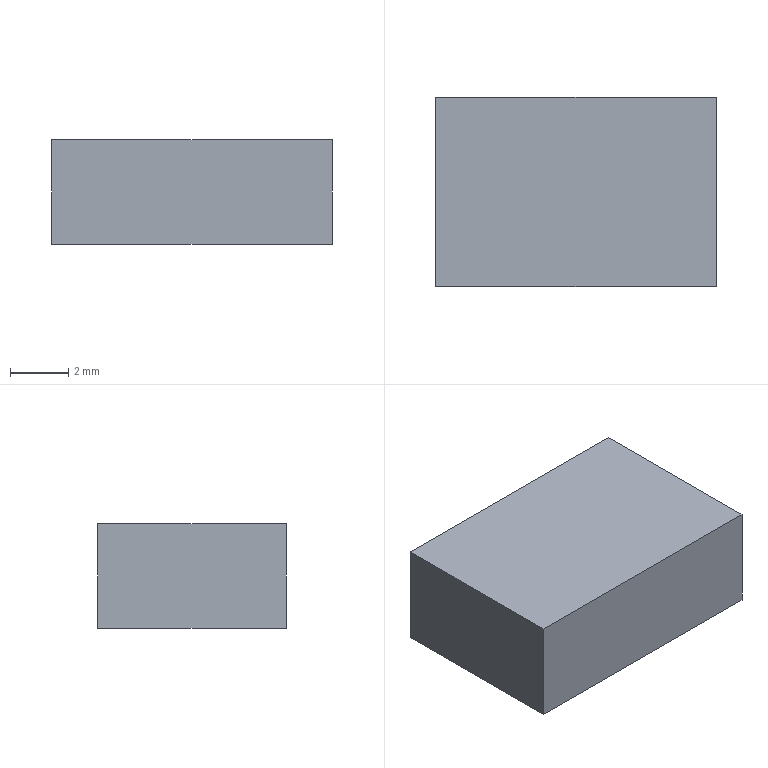Part | STEP file | RJ-USIO-V1_2-220411_28 | 1 solid | 6 faces | box 9.65 x 6.5 x 3.6 mm | volume 225.813 mm3 | plane 6
STEP:
#1=CARTESIAN_POINT('',(0.,0.,0.));
#2=DIRECTION('',(0.,0.,1.));
#3=DIRECTION('',(1.,0.,0.));
#4=AXIS2_PLACEMENT_3D('',#1,#2,#3);
#5=CARTESIAN_POINT('',(20.175,71.2,3.583));
#6=VERTEX_POINT('',#5);
#7=CARTESIAN_POINT('',(20.175,77.7,3.583));
#8=VERTEX_POINT('',#7);
#9=CARTESIAN_POINT('',(20.175,71.2,3.583));
#10=DIRECTION('',(0.,1.,0.));
#11=VECTOR('',#10,1.);
#12=LINE('',#9,#11);
#13=CARTESIAN_POINT('',(20.175,77.7,3.583));
#14=DIRECTION('',(0.,0.,-1.));
#15=DIRECTION('',(1.,0.,0.));
#16=AXIS2_PLACEMENT_3D('',#13,#14,#15);
#17=PLANE('',#16);
#18=CARTESIAN_POINT('',(0.,6.5));
#19=DIRECTION('',(0.,-1.));
#20=VECTOR('',#19,1.);
#21=LINE('',#18,#20);
#22=(GEOMETRIC_REPRESENTATION_CONTEXT(2)PARAMETRIC_REPRESENTATION_CONTEXT()REPRESENTATION_CONTEXT('',''));
#23=DEFINITIONAL_REPRESENTATION('',(#21),#22);
#24=PCURVE('',#17,#23);
#25=CARTESIAN_POINT('',(20.175,77.7,-0.01718));
#26=DIRECTION('',(1.,0.,0.));
#27=DIRECTION('',(0.,1.,0.));
#28=AXIS2_PLACEMENT_3D('',#25,#26,#27);
#29=PLANE('',#28);
#30=CARTESIAN_POINT('',(-6.5,3.6));
#31=DIRECTION('',(1.,0.));
#32=VECTOR('',#31,1.);
#33=LINE('',#30,#32);
#34=(GEOMETRIC_REPRESENTATION_CONTEXT(2)PARAMETRIC_REPRESENTATION_CONTEXT()REPRESENTATION_CONTEXT('',''));
#35=DEFINITIONAL_REPRESENTATION('',(#33),#34);
#36=PCURVE('',#29,#35);
#37=SURFACE_CURVE('',#12,(#24,#36),.PCURVE_S1.);
#38=EDGE_CURVE('',#6,#8,#37,.T.);
#39=ORIENTED_EDGE('',*,*,#38,.T.);
#40=CARTESIAN_POINT('',(29.825,77.7,3.583));
#41=VERTEX_POINT('',#40);
#42=CARTESIAN_POINT('',(20.175,77.7,3.583));
#43=DIRECTION('',(1.,0.,0.));
#44=VECTOR('',#43,1.);
#45=LINE('',#42,#44);
#46=CARTESIAN_POINT('',(0.,0.));
#47=DIRECTION('',(1.,0.));
#48=VECTOR('',#47,1.);
#49=LINE('',#46,#48);
#50=(GEOMETRIC_REPRESENTATION_CONTEXT(2)PARAMETRIC_REPRESENTATION_CONTEXT()REPRESENTATION_CONTEXT('',''));
#51=DEFINITIONAL_REPRESENTATION('',(#49),#50);
#52=PCURVE('',#17,#51);
#53=CARTESIAN_POINT('',(29.825,77.7,-0.01718));
#54=DIRECTION('',(0.,-1.,0.));
#55=DIRECTION('',(1.,0.,0.));
#56=AXIS2_PLACEMENT_3D('',#53,#54,#55);
#57=PLANE('',#56);
#58=CARTESIAN_POINT('',(-9.65,3.6));
#59=DIRECTION('',(1.,0.));
#60=VECTOR('',#59,1.);
#61=LINE('',#58,#60);
#62=(GEOMETRIC_REPRESENTATION_CONTEXT(2)PARAMETRIC_REPRESENTATION_CONTEXT()REPRESENTATION_CONTEXT('',''));
#63=DEFINITIONAL_REPRESENTATION('',(#61),#62);
#64=PCURVE('',#57,#63);
#65=SURFACE_CURVE('',#45,(#52,#64),.PCURVE_S1.);
#66=EDGE_CURVE('',#8,#41,#65,.T.);
#67=ORIENTED_EDGE('',*,*,#66,.T.);
#68=CARTESIAN_POINT('',(29.825,71.2,3.583));
#69=VERTEX_POINT('',#68);
#70=CARTESIAN_POINT('',(29.825,77.7,3.583));
#71=DIRECTION('',(0.,-1.,0.));
#72=VECTOR('',#71,1.);
#73=LINE('',#70,#72);
#74=CARTESIAN_POINT('',(9.65,0.));
#75=DIRECTION('',(0.,1.));
#76=VECTOR('',#75,1.);
#77=LINE('',#74,#76);
#78=(GEOMETRIC_REPRESENTATION_CONTEXT(2)PARAMETRIC_REPRESENTATION_CONTEXT()REPRESENTATION_CONTEXT('',''));
#79=DEFINITIONAL_REPRESENTATION('',(#77),#78);
#80=PCURVE('',#17,#79);
#81=CARTESIAN_POINT('',(29.825,71.2,-0.01718));
#82=DIRECTION('',(-1.,0.,0.));
#83=DIRECTION('',(0.,-1.,0.));
#84=AXIS2_PLACEMENT_3D('',#81,#82,#83);
#85=PLANE('',#84);
#86=CARTESIAN_POINT('',(-6.5,3.6));
#87=DIRECTION('',(1.,0.));
#88=VECTOR('',#87,1.);
#89=LINE('',#86,#88);
#90=(GEOMETRIC_REPRESENTATION_CONTEXT(2)PARAMETRIC_REPRESENTATION_CONTEXT()REPRESENTATION_CONTEXT('',''));
#91=DEFINITIONAL_REPRESENTATION('',(#89),#90);
#92=PCURVE('',#85,#91);
#93=SURFACE_CURVE('',#73,(#80,#92),.PCURVE_S1.);
#94=EDGE_CURVE('',#41,#69,#93,.T.);
#95=ORIENTED_EDGE('',*,*,#94,.T.);
#96=CARTESIAN_POINT('',(29.825,71.2,3.583));
#97=DIRECTION('',(-1.,0.,0.));
#98=VECTOR('',#97,1.);
#99=LINE('',#96,#98);
#100=CARTESIAN_POINT('',(9.65,6.5));
#101=DIRECTION('',(-1.,0.));
#102=VECTOR('',#101,1.);
#103=LINE('',#100,#102);
#104=(GEOMETRIC_REPRESENTATION_CONTEXT(2)PARAMETRIC_REPRESENTATION_CONTEXT()REPRESENTATION_CONTEXT('',''));
#105=DEFINITIONAL_REPRESENTATION('',(#103),#104);
#106=PCURVE('',#17,#105);
#107=CARTESIAN_POINT('',(20.175,71.2,-0.01718));
#108=DIRECTION('',(0.,1.,0.));
#109=DIRECTION('',(-1.,0.,0.));
#110=AXIS2_PLACEMENT_3D('',#107,#108,#109);
#111=PLANE('',#110);
#112=CARTESIAN_POINT('',(-9.65,3.6));
#113=DIRECTION('',(1.,0.));
#114=VECTOR('',#113,1.);
#115=LINE('',#112,#114);
#116=(GEOMETRIC_REPRESENTATION_CONTEXT(2)PARAMETRIC_REPRESENTATION_CONTEXT()REPRESENTATION_CONTEXT('',''));
#117=DEFINITIONAL_REPRESENTATION('',(#115),#116);
#118=PCURVE('',#111,#117);
#119=SURFACE_CURVE('',#99,(#106,#118),.PCURVE_S1.);
#120=EDGE_CURVE('',#69,#6,#119,.T.);
#121=ORIENTED_EDGE('',*,*,#120,.T.);
#122=EDGE_LOOP('',(#39,#67,#95,#121));
#123=FACE_BOUND('',#122,.F.);
#124=ADVANCED_FACE('',(#123),#17,.F.);
#125=CARTESIAN_POINT('',(20.175,71.2,-0.01718));
#126=VERTEX_POINT('',#125);
#127=CARTESIAN_POINT('',(20.175,77.7,-0.01718));
#128=VERTEX_POINT('',#127);
#129=CARTESIAN_POINT('',(20.175,71.2,-0.01718));
#130=DIRECTION('',(0.,1.,0.));
#131=VECTOR('',#130,1.);
#132=LINE('',#129,#131);
#133=CARTESIAN_POINT('',(-6.5,0.));
#134=DIRECTION('',(1.,0.));
#135=VECTOR('',#134,1.);
#136=LINE('',#133,#135);
#137=(GEOMETRIC_REPRESENTATION_CONTEXT(2)PARAMETRIC_REPRESENTATION_CONTEXT()REPRESENTATION_CONTEXT('',''));
#138=DEFINITIONAL_REPRESENTATION('',(#136),#137);
#139=PCURVE('',#29,#138);
#140=CARTESIAN_POINT('',(20.175,77.7,-0.01718));
#141=DIRECTION('',(0.,0.,-1.));
#142=DIRECTION('',(1.,0.,0.));
#143=AXIS2_PLACEMENT_3D('',#140,#141,#142);
#144=PLANE('',#143);
#145=CARTESIAN_POINT('',(0.,6.5));
#146=DIRECTION('',(0.,-1.));
#147=VECTOR('',#146,1.);
#148=LINE('',#145,#147);
#149=(GEOMETRIC_REPRESENTATION_CONTEXT(2)PARAMETRIC_REPRESENTATION_CONTEXT()REPRESENTATION_CONTEXT('',''));
#150=DEFINITIONAL_REPRESENTATION('',(#148),#149);
#151=PCURVE('',#144,#150);
#152=SURFACE_CURVE('',#132,(#139,#151),.PCURVE_S1.);
#153=EDGE_CURVE('',#126,#128,#152,.T.);
#154=ORIENTED_EDGE('',*,*,#153,.T.);
#155=CARTESIAN_POINT('',(20.175,77.7,3.583));
#156=DIRECTION('',(0.,0.,-1.));
#157=VECTOR('',#156,1.);
#158=LINE('',#155,#157);
#159=CARTESIAN_POINT('',(0.,3.6));
#160=DIRECTION('',(0.,-1.));
#161=VECTOR('',#160,1.);
#162=LINE('',#159,#161);
#163=(GEOMETRIC_REPRESENTATION_CONTEXT(2)PARAMETRIC_REPRESENTATION_CONTEXT()REPRESENTATION_CONTEXT('',''));
#164=DEFINITIONAL_REPRESENTATION('',(#162),#163);
#165=PCURVE('',#29,#164);
#166=CARTESIAN_POINT('',(-9.65,3.6));
#167=DIRECTION('',(0.,-1.));
#168=VECTOR('',#167,1.);
#169=LINE('',#166,#168);
#170=(GEOMETRIC_REPRESENTATION_CONTEXT(2)PARAMETRIC_REPRESENTATION_CONTEXT()REPRESENTATION_CONTEXT('',''));
#171=DEFINITIONAL_REPRESENTATION('',(#169),#170);
#172=PCURVE('',#57,#171);
#173=SURFACE_CURVE('',#158,(#165,#172),.PCURVE_S1.);
#174=EDGE_CURVE('',#8,#128,#173,.T.);
#175=ORIENTED_EDGE('',*,*,#174,.F.);
#176=ORIENTED_EDGE('',*,*,#38,.F.);
#177=CARTESIAN_POINT('',(20.175,71.2,3.583));
#178=DIRECTION('',(0.,0.,-1.));
#179=VECTOR('',#178,1.);
#180=LINE('',#177,#179);
#181=CARTESIAN_POINT('',(-6.5,3.6));
#182=DIRECTION('',(0.,-1.));
#183=VECTOR('',#182,1.);
#184=LINE('',#181,#183);
#185=(GEOMETRIC_REPRESENTATION_CONTEXT(2)PARAMETRIC_REPRESENTATION_CONTEXT()REPRESENTATION_CONTEXT('',''));
#186=DEFINITIONAL_REPRESENTATION('',(#184),#185);
#187=PCURVE('',#29,#186);
#188=CARTESIAN_POINT('',(0.,3.6));
#189=DIRECTION('',(0.,-1.));
#190=VECTOR('',#189,1.);
#191=LINE('',#188,#190);
#192=(GEOMETRIC_REPRESENTATION_CONTEXT(2)PARAMETRIC_REPRESENTATION_CONTEXT()REPRESENTATION_CONTEXT('',''));
#193=DEFINITIONAL_REPRESENTATION('',(#191),#192);
#194=PCURVE('',#111,#193);
#195=SURFACE_CURVE('',#180,(#187,#194),.PCURVE_S1.);
#196=EDGE_CURVE('',#6,#126,#195,.T.);
#197=ORIENTED_EDGE('',*,*,#196,.T.);
#198=EDGE_LOOP('',(#154,#175,#176,#197));
#199=FACE_BOUND('',#198,.F.);
#200=ADVANCED_FACE('',(#199),#29,.F.);
#201=CARTESIAN_POINT('',(29.825,77.7,-0.01718));
#202=VERTEX_POINT('',#201);
#203=CARTESIAN_POINT('',(20.175,77.7,-0.01718));
#204=DIRECTION('',(1.,0.,0.));
#205=VECTOR('',#204,1.);
#206=LINE('',#203,#205);
#207=CARTESIAN_POINT('',(0.,0.));
#208=DIRECTION('',(1.,0.));
#209=VECTOR('',#208,1.);
#210=LINE('',#207,#209);
#211=(GEOMETRIC_REPRESENTATION_CONTEXT(2)PARAMETRIC_REPRESENTATION_CONTEXT()REPRESENTATION_CONTEXT('',''));
#212=DEFINITIONAL_REPRESENTATION('',(#210),#211);
#213=PCURVE('',#144,#212);
#214=CARTESIAN_POINT('',(-9.65,0.));
#215=DIRECTION('',(1.,0.));
#216=VECTOR('',#215,1.);
#217=LINE('',#214,#216);
#218=(GEOMETRIC_REPRESENTATION_CONTEXT(2)PARAMETRIC_REPRESENTATION_CONTEXT()REPRESENTATION_CONTEXT('',''));
#219=DEFINITIONAL_REPRESENTATION('',(#217),#218);
#220=PCURVE('',#57,#219);
#221=SURFACE_CURVE('',#206,(#213,#220),.PCURVE_S1.);
#222=EDGE_CURVE('',#128,#202,#221,.T.);
#223=ORIENTED_EDGE('',*,*,#222,.F.);
#224=ORIENTED_EDGE('',*,*,#153,.F.);
#225=CARTESIAN_POINT('',(29.825,71.2,-0.01718));
#226=VERTEX_POINT('',#225);
#227=CARTESIAN_POINT('',(29.825,71.2,-0.01718));
#228=DIRECTION('',(-1.,0.,0.));
#229=VECTOR('',#228,1.);
#230=LINE('',#227,#229);
#231=CARTESIAN_POINT('',(9.65,6.5));
#232=DIRECTION('',(-1.,0.));
#233=VECTOR('',#232,1.);
#234=LINE('',#231,#233);
#235=(GEOMETRIC_REPRESENTATION_CONTEXT(2)PARAMETRIC_REPRESENTATION_CONTEXT()REPRESENTATION_CONTEXT('',''));
#236=DEFINITIONAL_REPRESENTATION('',(#234),#235);
#237=PCURVE('',#144,#236);
#238=CARTESIAN_POINT('',(-9.65,0.));
#239=DIRECTION('',(1.,0.));
#240=VECTOR('',#239,1.);
#241=LINE('',#238,#240);
#242=(GEOMETRIC_REPRESENTATION_CONTEXT(2)PARAMETRIC_REPRESENTATION_CONTEXT()REPRESENTATION_CONTEXT('',''));
#243=DEFINITIONAL_REPRESENTATION('',(#241),#242);
#244=PCURVE('',#111,#243);
#245=SURFACE_CURVE('',#230,(#237,#244),.PCURVE_S1.);
#246=EDGE_CURVE('',#226,#126,#245,.T.);
#247=ORIENTED_EDGE('',*,*,#246,.F.);
#248=CARTESIAN_POINT('',(29.825,77.7,-0.01718));
#249=DIRECTION('',(0.,-1.,0.));
#250=VECTOR('',#249,1.);
#251=LINE('',#248,#250);
#252=CARTESIAN_POINT('',(9.65,0.));
#253=DIRECTION('',(0.,1.));
#254=VECTOR('',#253,1.);
#255=LINE('',#252,#254);
#256=(GEOMETRIC_REPRESENTATION_CONTEXT(2)PARAMETRIC_REPRESENTATION_CONTEXT()REPRESENTATION_CONTEXT('',''));
#257=DEFINITIONAL_REPRESENTATION('',(#255),#256);
#258=PCURVE('',#144,#257);
#259=CARTESIAN_POINT('',(-6.5,0.));
#260=DIRECTION('',(1.,0.));
#261=VECTOR('',#260,1.);
#262=LINE('',#259,#261);
#263=(GEOMETRIC_REPRESENTATION_CONTEXT(2)PARAMETRIC_REPRESENTATION_CONTEXT()REPRESENTATION_CONTEXT('',''));
#264=DEFINITIONAL_REPRESENTATION('',(#262),#263);
#265=PCURVE('',#85,#264);
#266=SURFACE_CURVE('',#251,(#258,#265),.PCURVE_S1.);
#267=EDGE_CURVE('',#202,#226,#266,.T.);
#268=ORIENTED_EDGE('',*,*,#267,.F.);
#269=EDGE_LOOP('',(#223,#224,#247,#268));
#270=FACE_BOUND('',#269,.F.);
#271=ADVANCED_FACE('',(#270),#144,.T.);
#272=ORIENTED_EDGE('',*,*,#222,.T.);
#273=CARTESIAN_POINT('',(29.825,77.7,3.583));
#274=DIRECTION('',(0.,0.,-1.));
#275=VECTOR('',#274,1.);
#276=LINE('',#273,#275);
#277=CARTESIAN_POINT('',(0.,3.6));
#278=DIRECTION('',(0.,-1.));
#279=VECTOR('',#278,1.);
#280=LINE('',#277,#279);
#281=(GEOMETRIC_REPRESENTATION_CONTEXT(2)PARAMETRIC_REPRESENTATION_CONTEXT()REPRESENTATION_CONTEXT('',''));
#282=DEFINITIONAL_REPRESENTATION('',(#280),#281);
#283=PCURVE('',#57,#282);
#284=CARTESIAN_POINT('',(-6.5,3.6));
#285=DIRECTION('',(0.,-1.));
#286=VECTOR('',#285,1.);
#287=LINE('',#284,#286);
#288=(GEOMETRIC_REPRESENTATION_CONTEXT(2)PARAMETRIC_REPRESENTATION_CONTEXT()REPRESENTATION_CONTEXT('',''));
#289=DEFINITIONAL_REPRESENTATION('',(#287),#288);
#290=PCURVE('',#85,#289);
#291=SURFACE_CURVE('',#276,(#283,#290),.PCURVE_S1.);
#292=EDGE_CURVE('',#41,#202,#291,.T.);
#293=ORIENTED_EDGE('',*,*,#292,.F.);
#294=ORIENTED_EDGE('',*,*,#66,.F.);
#295=ORIENTED_EDGE('',*,*,#174,.T.);
#296=EDGE_LOOP('',(#272,#293,#294,#295));
#297=FACE_BOUND('',#296,.F.);
#298=ADVANCED_FACE('',(#297),#57,.F.);
#299=ORIENTED_EDGE('',*,*,#267,.T.);
#300=CARTESIAN_POINT('',(29.825,71.2,3.583));
#301=DIRECTION('',(0.,0.,-1.));
#302=VECTOR('',#301,1.);
#303=LINE('',#300,#302);
#304=CARTESIAN_POINT('',(0.,3.6));
#305=DIRECTION('',(0.,-1.));
#306=VECTOR('',#305,1.);
#307=LINE('',#304,#306);
#308=(GEOMETRIC_REPRESENTATION_CONTEXT(2)PARAMETRIC_REPRESENTATION_CONTEXT()REPRESENTATION_CONTEXT('',''));
#309=DEFINITIONAL_REPRESENTATION('',(#307),#308);
#310=PCURVE('',#85,#309);
#311=CARTESIAN_POINT('',(-9.65,3.6));
#312=DIRECTION('',(0.,-1.));
#313=VECTOR('',#312,1.);
#314=LINE('',#311,#313);
#315=(GEOMETRIC_REPRESENTATION_CONTEXT(2)PARAMETRIC_REPRESENTATION_CONTEXT()REPRESENTATION_CONTEXT('',''));
#316=DEFINITIONAL_REPRESENTATION('',(#314),#315);
#317=PCURVE('',#111,#316);
#318=SURFACE_CURVE('',#303,(#310,#317),.PCURVE_S1.);
#319=EDGE_CURVE('',#69,#226,#318,.T.);
#320=ORIENTED_EDGE('',*,*,#319,.F.);
#321=ORIENTED_EDGE('',*,*,#94,.F.);
#322=ORIENTED_EDGE('',*,*,#292,.T.);
#323=EDGE_LOOP('',(#299,#320,#321,#322));
#324=FACE_BOUND('',#323,.F.);
#325=ADVANCED_FACE('',(#324),#85,.F.);
#326=ORIENTED_EDGE('',*,*,#246,.T.);
#327=ORIENTED_EDGE('',*,*,#196,.F.);
#328=ORIENTED_EDGE('',*,*,#120,.F.);
#329=ORIENTED_EDGE('',*,*,#319,.T.);
#330=EDGE_LOOP('',(#326,#327,#328,#329));
#331=FACE_BOUND('',#330,.F.);
#332=ADVANCED_FACE('',(#331),#111,.F.);
#333=CLOSED_SHELL('',(#124,#200,#271,#298,#325,#332));
#334=MANIFOLD_SOLID_BREP('',#333);
#335=(LENGTH_UNIT()NAMED_UNIT(*)SI_UNIT(.MILLI.,.METRE.));
#336=UNCERTAINTY_MEASURE_WITH_UNIT(LENGTH_MEASURE(0.0000001),#335,'','');
#337=(NAMED_UNIT(*)PLANE_ANGLE_UNIT()SI_UNIT($,.RADIAN.));
#338=(NAMED_UNIT(*)SI_UNIT($,.STERADIAN.)SOLID_ANGLE_UNIT());
#339=(GEOMETRIC_REPRESENTATION_CONTEXT(3)GLOBAL_UNCERTAINTY_ASSIGNED_CONTEXT((#336))GLOBAL_UNIT_ASSIGNED_CONTEXT((#335,#337,#338))REPRESENTATION_CONTEXT('',''));
#340=ADVANCED_BREP_SHAPE_REPRESENTATION('',(#4,#334),#339);